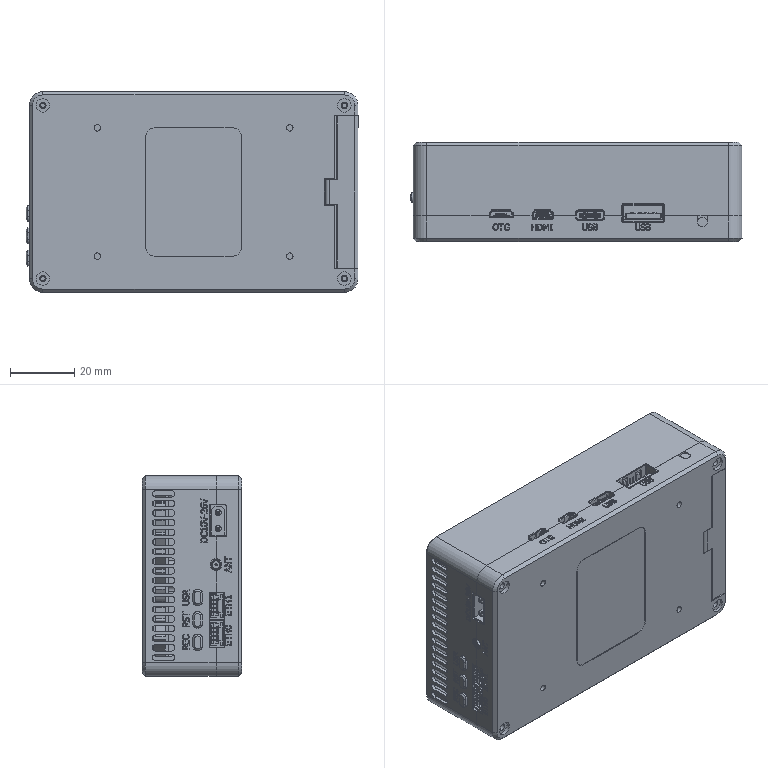Part | SolidWorks | features BaseBody 27 | 27 solids | 8359 faces | volume 32010 mm3 | plane 6289 | cylinder 1264 | spline 709 | cone 78 | torus 15 | sphere 4 | commonest cylinder face diameters 0.6 x202 0.3 x195 0.2 x103 0.4 x81 2 x72 1 x70